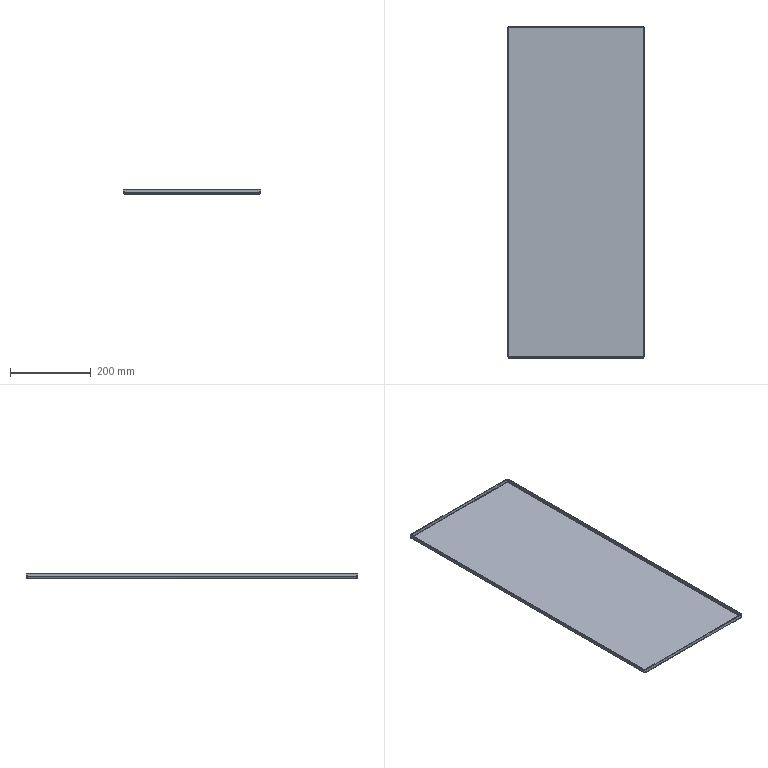Part | SolidWorks | features BaseBody 1 | 1 solid | 38 faces | box 340 x 820 x 10 mm | volume 590888 mm3 | plane 22 | cylinder 8 | spline 8 | commonest cylinder face diameters 1.473 x4 5.473 x4
STEP:
#1=CARTESIAN_POINT('',(-167.263,-407.263,-2.));
#2=VERTEX_POINT('',#1);
#3=CARTESIAN_POINT('',(-167.263,407.263,-2.));
#4=VERTEX_POINT('',#3);
#5=CARTESIAN_POINT('',(-167.263,0.,-2.));
#6=DIRECTION('',(0.,1.,0.));
#7=VECTOR('',#6,1000.);
#8=LINE('',#5,#7);
#9=EDGE_CURVE('',#2,#4,#8,.T.);
#10=ORIENTED_EDGE('',*,*,#9,.T.);
#11=CARTESIAN_POINT('',(167.263,407.263,-2.));
#12=VERTEX_POINT('',#11);
#13=CARTESIAN_POINT('',(0.,407.263,-2.));
#14=DIRECTION('',(1.,0.,0.));
#15=VECTOR('',#14,1000.);
#16=LINE('',#13,#15);
#17=EDGE_CURVE('',#4,#12,#16,.T.);
#18=ORIENTED_EDGE('',*,*,#17,.T.);
#19=CARTESIAN_POINT('',(167.263,-407.263,-2.));
#20=VERTEX_POINT('',#19);
#21=CARTESIAN_POINT('',(167.263,0.,-2.));
#22=DIRECTION('',(0.,-1.,0.));
#23=VECTOR('',#22,1000.);
#24=LINE('',#21,#23);
#25=EDGE_CURVE('',#12,#20,#24,.T.);
#26=ORIENTED_EDGE('',*,*,#25,.T.);
#27=CARTESIAN_POINT('',(0.,-407.263,-2.));
#28=DIRECTION('',(-1.,0.,0.));
#29=VECTOR('',#28,1000.);
#30=LINE('',#27,#29);
#31=EDGE_CURVE('',#20,#2,#30,.T.);
#32=ORIENTED_EDGE('',*,*,#31,.T.);
#33=EDGE_LOOP('',(#10,#18,#26,#32));
#34=FACE_OUTER_BOUND('',#33,.T.);
#35=CARTESIAN_POINT('',(167.263,-407.263,-2.));
#36=DIRECTION('',(0.,0.,-1.));
#37=DIRECTION('',(-1.,0.,0.));
#38=AXIS2_PLACEMENT_3D('',#35,#36,#37);
#39=PLANE('',#38);
#40=ADVANCED_FACE('',(#34),#39,.T.);
#41=CARTESIAN_POINT('',(-167.293,410.,0.7366));
#42=VERTEX_POINT('',#41);
#43=CARTESIAN_POINT('',(-167.293,410.,0.7366));
#44=CARTESIAN_POINT('',(-167.29,410.,0.3784));
#45=CARTESIAN_POINT('',(-167.288,409.929,0.0203));
#46=CARTESIAN_POINT('',(-167.283,409.655,-0.6416));
#47=CARTESIAN_POINT('',(-167.281,409.452,-0.9452));
#48=CARTESIAN_POINT('',(-167.276,408.945,-1.452));
#49=CARTESIAN_POINT('',(-167.273,408.642,-1.655));
#50=CARTESIAN_POINT('',(-167.268,407.98,-1.929));
#51=CARTESIAN_POINT('',(-167.266,407.622,-2.));
#52=CARTESIAN_POINT('',(-167.263,407.263,-2.));
#53=B_SPLINE_CURVE_WITH_KNOTS('',3,(#43,#44,#45,#46,#47,#48,#49,#50,#51,#52),.UNSPECIFIED.,.F.,.F.,(4,2,2,2,4),(0.,0.25,0.5,0.75,1.),.UNSPECIFIED.);
#54=EDGE_CURVE('',#42,#4,#53,.T.);
#55=ORIENTED_EDGE('',*,*,#54,.F.);
#56=CARTESIAN_POINT('',(167.293,410.,0.7366));
#57=VERTEX_POINT('',#56);
#58=CARTESIAN_POINT('',(0.,410.,0.7366));
#59=DIRECTION('',(-1.,0.,0.));
#60=VECTOR('',#59,1000.);
#61=LINE('',#58,#60);
#62=EDGE_CURVE('',#57,#42,#61,.T.);
#63=ORIENTED_EDGE('',*,*,#62,.F.);
#64=CARTESIAN_POINT('',(167.263,407.263,-2.));
#65=CARTESIAN_POINT('',(167.266,407.622,-2.));
#66=CARTESIAN_POINT('',(167.268,407.98,-1.929));
#67=CARTESIAN_POINT('',(167.273,408.642,-1.655));
#68=CARTESIAN_POINT('',(167.276,408.945,-1.452));
#69=CARTESIAN_POINT('',(167.281,409.452,-0.9452));
#70=CARTESIAN_POINT('',(167.283,409.655,-0.6416));
#71=CARTESIAN_POINT('',(167.288,409.929,0.0203));
#72=CARTESIAN_POINT('',(167.29,410.,0.3784));
#73=CARTESIAN_POINT('',(167.293,410.,0.7366));
#74=B_SPLINE_CURVE_WITH_KNOTS('',3,(#64,#65,#66,#67,#68,#69,#70,#71,#72,#73),.UNSPECIFIED.,.F.,.F.,(4,2,2,2,4),(0.,0.25,0.5,0.75,1.),.UNSPECIFIED.);
#75=EDGE_CURVE('',#12,#57,#74,.T.);
#76=ORIENTED_EDGE('',*,*,#75,.F.);
#77=ORIENTED_EDGE('',*,*,#17,.F.);
#78=EDGE_LOOP('',(#55,#63,#76,#77));
#79=FACE_OUTER_BOUND('',#78,.T.);
#80=CARTESIAN_POINT('',(169.3,407.263,0.7366));
#81=DIRECTION('',(-1.,0.,0.));
#82=DIRECTION('',(0.,0.,1.));
#83=AXIS2_PLACEMENT_3D('',#80,#81,#82);
#84=CYLINDRICAL_SURFACE('',#83,2.737);
#85=ADVANCED_FACE('',(#79),#84,.T.);
#86=CARTESIAN_POINT('',(-170.,-407.293,0.7366));
#87=VERTEX_POINT('',#86);
#88=CARTESIAN_POINT('',(-170.,-407.293,0.7366));
#89=CARTESIAN_POINT('',(-170.,-407.29,0.3784));
#90=CARTESIAN_POINT('',(-169.929,-407.288,0.0203));
#91=CARTESIAN_POINT('',(-169.655,-407.283,-0.6416));
#92=CARTESIAN_POINT('',(-169.452,-407.281,-0.9452));
#93=CARTESIAN_POINT('',(-168.945,-407.276,-1.452));
#94=CARTESIAN_POINT('',(-168.642,-407.273,-1.655));
#95=CARTESIAN_POINT('',(-167.98,-407.268,-1.929));
#96=CARTESIAN_POINT('',(-167.622,-407.266,-2.));
#97=CARTESIAN_POINT('',(-167.263,-407.263,-2.));
#98=B_SPLINE_CURVE_WITH_KNOTS('',3,(#88,#89,#90,#91,#92,#93,#94,#95,#96,#97),.UNSPECIFIED.,.F.,.F.,(4,2,2,2,4),(0.,0.25,0.5,0.75,1.),.UNSPECIFIED.);
#99=EDGE_CURVE('',#87,#2,#98,.T.);
#100=ORIENTED_EDGE('',*,*,#99,.F.);
#101=CARTESIAN_POINT('',(-170.,407.293,0.7366));
#102=VERTEX_POINT('',#101);
#103=CARTESIAN_POINT('',(-170.,0.,0.7366));
#104=DIRECTION('',(0.,-1.,0.));
#105=VECTOR('',#104,1000.);
#106=LINE('',#103,#105);
#107=EDGE_CURVE('',#102,#87,#106,.T.);
#108=ORIENTED_EDGE('',*,*,#107,.F.);
#109=CARTESIAN_POINT('',(-167.263,407.263,-2.));
#110=CARTESIAN_POINT('',(-167.622,407.266,-2.));
#111=CARTESIAN_POINT('',(-167.98,407.268,-1.929));
#112=CARTESIAN_POINT('',(-168.642,407.273,-1.655));
#113=CARTESIAN_POINT('',(-168.945,407.276,-1.452));
#114=CARTESIAN_POINT('',(-169.452,407.281,-0.9452));
#115=CARTESIAN_POINT('',(-169.655,407.283,-0.6416));
#116=CARTESIAN_POINT('',(-169.929,407.288,0.0203));
#117=CARTESIAN_POINT('',(-170.,407.29,0.3784));
#118=CARTESIAN_POINT('',(-170.,407.293,0.7366));
#119=B_SPLINE_CURVE_WITH_KNOTS('',3,(#109,#110,#111,#112,#113,#114,#115,#116,#117,#118),.UNSPECIFIED.,.F.,.F.,(4,2,2,2,4),(0.,0.25,0.5,0.75,1.),.UNSPECIFIED.);
#120=EDGE_CURVE('',#4,#102,#119,.T.);
#121=ORIENTED_EDGE('',*,*,#120,.F.);
#122=ORIENTED_EDGE('',*,*,#9,.F.);
#123=EDGE_LOOP('',(#100,#108,#121,#122));
#124=FACE_OUTER_BOUND('',#123,.T.);
#125=CARTESIAN_POINT('',(-167.263,412.18,0.7366));
#126=DIRECTION('',(0.,-1.,0.));
#127=DIRECTION('',(0.,0.,-1.));
#128=AXIS2_PLACEMENT_3D('',#125,#126,#127);
#129=CYLINDRICAL_SURFACE('',#128,2.737);
#130=ADVANCED_FACE('',(#124),#129,.T.);
#131=CARTESIAN_POINT('',(167.293,-410.,0.7366));
#132=VERTEX_POINT('',#131);
#133=CARTESIAN_POINT('',(167.293,-410.,0.7366));
#134=CARTESIAN_POINT('',(167.29,-410.,0.3784));
#135=CARTESIAN_POINT('',(167.288,-409.929,0.0203));
#136=CARTESIAN_POINT('',(167.283,-409.655,-0.6416));
#137=CARTESIAN_POINT('',(167.281,-409.452,-0.9452));
#138=CARTESIAN_POINT('',(167.276,-408.945,-1.452));
#139=CARTESIAN_POINT('',(167.273,-408.642,-1.655));
#140=CARTESIAN_POINT('',(167.268,-407.98,-1.929));
#141=CARTESIAN_POINT('',(167.266,-407.622,-2.));
#142=CARTESIAN_POINT('',(167.263,-407.263,-2.));
#143=B_SPLINE_CURVE_WITH_KNOTS('',3,(#133,#134,#135,#136,#137,#138,#139,#140,#141,#142),.UNSPECIFIED.,.F.,.F.,(4,2,2,2,4),(0.,0.25,0.5,0.75,1.),.UNSPECIFIED.);
#144=EDGE_CURVE('',#132,#20,#143,.T.);
#145=ORIENTED_EDGE('',*,*,#144,.F.);
#146=CARTESIAN_POINT('',(-167.293,-410.,0.7366));
#147=VERTEX_POINT('',#146);
#148=CARTESIAN_POINT('',(0.,-410.,0.7366));
#149=DIRECTION('',(1.,0.,0.));
#150=VECTOR('',#149,1000.);
#151=LINE('',#148,#150);
#152=EDGE_CURVE('',#147,#132,#151,.T.);
#153=ORIENTED_EDGE('',*,*,#152,.F.);
#154=CARTESIAN_POINT('',(-167.263,-407.263,-2.));
#155=CARTESIAN_POINT('',(-167.266,-407.622,-2.));
#156=CARTESIAN_POINT('',(-167.268,-407.98,-1.929));
#157=CARTESIAN_POINT('',(-167.273,-408.642,-1.655));
#158=CARTESIAN_POINT('',(-167.276,-408.945,-1.452));
#159=CARTESIAN_POINT('',(-167.281,-409.452,-0.9452));
#160=CARTESIAN_POINT('',(-167.283,-409.655,-0.6416));
#161=CARTESIAN_POINT('',(-167.288,-409.929,0.0203));
#162=CARTESIAN_POINT('',(-167.29,-410.,0.3784));
#163=CARTESIAN_POINT('',(-167.293,-410.,0.7366));
#164=B_SPLINE_CURVE_WITH_KNOTS('',3,(#154,#155,#156,#157,#158,#159,#160,#161,#162,#163),.UNSPECIFIED.,.F.,.F.,(4,2,2,2,4),(0.,0.25,0.5,0.75,1.),.UNSPECIFIED.);
#165=EDGE_CURVE('',#2,#147,#164,.T.);
#166=ORIENTED_EDGE('',*,*,#165,.F.);
#167=ORIENTED_EDGE('',*,*,#31,.F.);
#168=EDGE_LOOP('',(#145,#153,#166,#167));
#169=FACE_OUTER_BOUND('',#168,.T.);
#170=CARTESIAN_POINT('',(-169.3,-407.263,0.7366));
#171=DIRECTION('',(1.,0.,0.));
#172=DIRECTION('',(0.,0.,-1.));
#173=AXIS2_PLACEMENT_3D('',#170,#171,#172);
#174=CYLINDRICAL_SURFACE('',#173,2.737);
#175=ADVANCED_FACE('',(#169),#174,.T.);
#176=CARTESIAN_POINT('',(170.,407.293,0.7366));
#177=VERTEX_POINT('',#176);
#178=CARTESIAN_POINT('',(170.,407.293,0.7366));
#179=CARTESIAN_POINT('',(170.,407.29,0.3784));
#180=CARTESIAN_POINT('',(169.929,407.288,0.0203));
#181=CARTESIAN_POINT('',(169.655,407.283,-0.6416));
#182=CARTESIAN_POINT('',(169.452,407.281,-0.9452));
#183=CARTESIAN_POINT('',(168.945,407.276,-1.452));
#184=CARTESIAN_POINT('',(168.642,407.273,-1.655));
#185=CARTESIAN_POINT('',(167.98,407.268,-1.929));
#186=CARTESIAN_POINT('',(167.622,407.266,-2.));
#187=CARTESIAN_POINT('',(167.263,407.263,-2.));
#188=B_SPLINE_CURVE_WITH_KNOTS('',3,(#178,#179,#180,#181,#182,#183,#184,#185,#186,#187),.UNSPECIFIED.,.F.,.F.,(4,2,2,2,4),(0.,0.25,0.5,0.75,1.),.UNSPECIFIED.);
#189=EDGE_CURVE('',#177,#12,#188,.T.);
#190=ORIENTED_EDGE('',*,*,#189,.F.);
#191=CARTESIAN_POINT('',(170.,-407.293,0.7366));
#192=VERTEX_POINT('',#191);
#193=CARTESIAN_POINT('',(170.,0.,0.7366));
#194=DIRECTION('',(0.,1.,0.));
#195=VECTOR('',#194,1000.);
#196=LINE('',#193,#195);
#197=EDGE_CURVE('',#192,#177,#196,.T.);
#198=ORIENTED_EDGE('',*,*,#197,.F.);
#199=CARTESIAN_POINT('',(167.263,-407.263,-2.));
#200=CARTESIAN_POINT('',(167.622,-407.266,-2.));
#201=CARTESIAN_POINT('',(167.98,-407.268,-1.929));
#202=CARTESIAN_POINT('',(168.642,-407.273,-1.655));
#203=CARTESIAN_POINT('',(168.945,-407.276,-1.452));
#204=CARTESIAN_POINT('',(169.452,-407.281,-0.9452));
#205=CARTESIAN_POINT('',(169.655,-407.283,-0.6416));
#206=CARTESIAN_POINT('',(169.929,-407.288,0.0203));
#207=CARTESIAN_POINT('',(170.,-407.29,0.3784));
#208=CARTESIAN_POINT('',(170.,-407.293,0.7366));
#209=B_SPLINE_CURVE_WITH_KNOTS('',3,(#199,#200,#201,#202,#203,#204,#205,#206,#207,#208),.UNSPECIFIED.,.F.,.F.,(4,2,2,2,4),(0.,0.25,0.5,0.75,1.),.UNSPECIFIED.);
#210=EDGE_CURVE('',#20,#192,#209,.T.);
#211=ORIENTED_EDGE('',*,*,#210,.F.);
#212=ORIENTED_EDGE('',*,*,#25,.F.);
#213=EDGE_LOOP('',(#190,#198,#211,#212));
#214=FACE_OUTER_BOUND('',#213,.T.);
#215=CARTESIAN_POINT('',(167.263,-412.18,0.7366));
#216=DIRECTION('',(0.,1.,0.));
#217=DIRECTION('',(0.,0.,1.));
#218=AXIS2_PLACEMENT_3D('',#215,#216,#217);
#219=CYLINDRICAL_SURFACE('',#218,2.737);
#220=ADVANCED_FACE('',(#214),#219,.T.);
#221=CARTESIAN_POINT('',(-167.293,408.,0.7366));
#222=VERTEX_POINT('',#221);
#223=CARTESIAN_POINT('',(-167.293,409.,0.7366));
#224=DIRECTION('',(0.,-1.,0.));
#225=VECTOR('',#224,1000.);
#226=LINE('',#223,#225);
#227=EDGE_CURVE('',#42,#222,#226,.T.);
#228=ORIENTED_EDGE('',*,*,#227,.F.);
#229=ORIENTED_EDGE('',*,*,#54,.T.);
#230=CARTESIAN_POINT('',(-167.263,407.263,0.));
#231=VERTEX_POINT('',#230);
#232=CARTESIAN_POINT('',(-167.263,407.263,-1.));
#233=DIRECTION('',(0.,0.,-1.));
#234=VECTOR('',#233,1000.);
#235=LINE('',#232,#234);
#236=EDGE_CURVE('',#231,#4,#235,.T.);
#237=ORIENTED_EDGE('',*,*,#236,.F.);
#238=CARTESIAN_POINT('',(-167.293,408.,0.7366));
#239=CARTESIAN_POINT('',(-167.288,408.,0.5438));
#240=CARTESIAN_POINT('',(-167.283,407.921,0.3521));
#241=CARTESIAN_POINT('',(-167.273,407.648,0.07939));
#242=CARTESIAN_POINT('',(-167.268,407.456,0.));
#243=CARTESIAN_POINT('',(-167.263,407.263,0.));
#244=B_SPLINE_CURVE_WITH_KNOTS('',3,(#238,#239,#240,#241,#242,#243),.UNSPECIFIED.,.F.,.F.,(4,2,4),(0.,0.5,1.),.UNSPECIFIED.);
#245=EDGE_CURVE('',#222,#231,#244,.T.);
#246=ORIENTED_EDGE('',*,*,#245,.F.);
#247=EDGE_LOOP('',(#228,#229,#237,#246));
#248=FACE_OUTER_BOUND('',#247,.T.);
#249=CARTESIAN_POINT('',(-167.293,410.012,0.7366));
#250=CARTESIAN_POINT('',(-167.29,410.012,0.3767));
#251=CARTESIAN_POINT('',(-167.288,409.941,0.01711));
#252=CARTESIAN_POINT('',(-167.283,409.665,-0.6477));
#253=CARTESIAN_POINT('',(-167.281,409.462,-0.9527));
#254=CARTESIAN_POINT('',(-167.276,408.953,-1.462));
#255=CARTESIAN_POINT('',(-167.273,408.648,-1.665));
#256=CARTESIAN_POINT('',(-167.268,407.983,-1.941));
#257=CARTESIAN_POINT('',(-167.266,407.623,-2.012));
#258=CARTESIAN_POINT('',(-167.263,407.263,-2.012));
#259=CARTESIAN_POINT('',(-167.293,410.,0.7366));
#260=CARTESIAN_POINT('',(-167.29,410.,0.3783));
#261=CARTESIAN_POINT('',(-167.288,409.929,0.0203));
#262=CARTESIAN_POINT('',(-167.283,409.655,-0.6416));
#263=CARTESIAN_POINT('',(-167.281,409.452,-0.9452));
#264=CARTESIAN_POINT('',(-167.276,408.945,-1.452));
#265=CARTESIAN_POINT('',(-167.273,408.642,-1.655));
#266=CARTESIAN_POINT('',(-167.268,407.98,-1.929));
#267=CARTESIAN_POINT('',(-167.266,407.622,-2.));
#268=CARTESIAN_POINT('',(-167.263,407.263,-2.));
#269=CARTESIAN_POINT('',(-167.293,408.,0.7366));
#270=CARTESIAN_POINT('',(-167.29,408.,0.6402));
#271=CARTESIAN_POINT('',(-167.288,407.981,0.5438));
#272=CARTESIAN_POINT('',(-167.283,407.907,0.3656));
#273=CARTESIAN_POINT('',(-167.281,407.852,0.2839));
#274=CARTESIAN_POINT('',(-167.276,407.716,0.1476));
#275=CARTESIAN_POINT('',(-167.273,407.634,0.09297));
#276=CARTESIAN_POINT('',(-167.268,407.456,0.01917));
#277=CARTESIAN_POINT('',(-167.266,407.36,0.));
#278=CARTESIAN_POINT('',(-167.263,407.263,0.));
#279=CARTESIAN_POINT('',(-167.293,407.988,0.7366));
#280=CARTESIAN_POINT('',(-167.29,407.988,0.6417));
#281=CARTESIAN_POINT('',(-167.288,407.969,0.5469));
#282=CARTESIAN_POINT('',(-167.283,407.897,0.3717));
#283=CARTESIAN_POINT('',(-167.281,407.843,0.2913));
#284=CARTESIAN_POINT('',(-167.276,407.709,0.1572));
#285=CARTESIAN_POINT('',(-167.273,407.628,0.1035));
#286=CARTESIAN_POINT('',(-167.268,407.453,0.03088));
#287=CARTESIAN_POINT('',(-167.266,407.358,0.01202));
#288=CARTESIAN_POINT('',(-167.263,407.263,0.01202));
#289=B_SPLINE_SURFACE_WITH_KNOTS('',1,3,((#249,#250,#251,#252,#253,#254,#255,#256,#257,#258),(#259,#260,#261,#262,#263,#264,#265,#266,#267,#268),(#269,#270,#271,#272,#273,#274,#275,#276,#277,#278),(#279,#280,#281,#282,#283,#284,#285,#286,#287,#288)),.UNSPECIFIED.,.F.,.F.,.F.,(2,1,1,2),(4,2,2,2,4),(-0.006096,0.,1.,1.006),(0.,0.25,0.5,0.75,1.),.UNSPECIFIED.);
#290=ADVANCED_FACE('',(#248),#289,.F.);
#291=CARTESIAN_POINT('',(-167.293,410.,8.));
#292=VERTEX_POINT('',#291);
#293=CARTESIAN_POINT('',(-167.293,410.,4.368));
#294=DIRECTION('',(0.,0.,-1.));
#295=VECTOR('',#294,1000.);
#296=LINE('',#293,#295);
#297=EDGE_CURVE('',#292,#42,#296,.T.);
#298=ORIENTED_EDGE('',*,*,#297,.F.);
#299=CARTESIAN_POINT('',(167.293,410.,8.));
#300=VERTEX_POINT('',#299);
#301=CARTESIAN_POINT('',(0.,410.,8.));
#302=DIRECTION('',(-1.,0.,0.));
#303=VECTOR('',#302,1000.);
#304=LINE('',#301,#303);
#305=EDGE_CURVE('',#300,#292,#304,.T.);
#306=ORIENTED_EDGE('',*,*,#305,.F.);
#307=CARTESIAN_POINT('',(167.293,410.,4.368));
#308=DIRECTION('',(0.,0.,1.));
#309=VECTOR('',#308,1000.);
#310=LINE('',#307,#309);
#311=EDGE_CURVE('',#57,#300,#310,.T.);
#312=ORIENTED_EDGE('',*,*,#311,.F.);
#313=ORIENTED_EDGE('',*,*,#62,.T.);
#314=EDGE_LOOP('',(#298,#306,#312,#313));
#315=FACE_OUTER_BOUND('',#314,.T.);
#316=CARTESIAN_POINT('',(-167.293,410.,8.));
#317=DIRECTION('',(0.,-1.,0.));
#318=DIRECTION('',(0.,0.,-1.));
#319=AXIS2_PLACEMENT_3D('',#316,#317,#318);
#320=PLANE('',#319);
#321=ADVANCED_FACE('',(#315),#320,.F.);
#322=CARTESIAN_POINT('',(167.263,407.263,0.));
#323=VERTEX_POINT('',#322);
#324=CARTESIAN_POINT('',(167.293,408.,0.7366));
#325=VERTEX_POINT('',#324);
#326=CARTESIAN_POINT('',(167.263,407.263,0.));
#327=CARTESIAN_POINT('',(167.268,407.456,0.));
#328=CARTESIAN_POINT('',(167.273,407.648,0.07939));
#329=CARTESIAN_POINT('',(167.283,407.921,0.3521));
#330=CARTESIAN_POINT('',(167.288,408.,0.5438));
#331=CARTESIAN_POINT('',(167.293,408.,0.7366));
#332=B_SPLINE_CURVE_WITH_KNOTS('',3,(#326,#327,#328,#329,#330,#331),.UNSPECIFIED.,.F.,.F.,(4,2,4),(0.,0.5,1.),.UNSPECIFIED.);
#333=EDGE_CURVE('',#323,#325,#332,.T.);
#334=ORIENTED_EDGE('',*,*,#333,.F.);
#335=CARTESIAN_POINT('',(167.263,407.263,-1.));
#336=DIRECTION('',(0.,0.,1.));
#337=VECTOR('',#336,1000.);
#338=LINE('',#335,#337);
#339=EDGE_CURVE('',#12,#323,#338,.T.);
#340=ORIENTED_EDGE('',*,*,#339,.F.);
#341=ORIENTED_EDGE('',*,*,#75,.T.);
#342=CARTESIAN_POINT('',(167.293,409.,0.7366));
#343=DIRECTION('',(0.,1.,0.));
#344=VECTOR('',#343,1000.);
#345=LINE('',#342,#344);
#346=EDGE_CURVE('',#325,#57,#345,.T.);
#347=ORIENTED_EDGE('',*,*,#346,.F.);
#348=EDGE_LOOP('',(#334,#340,#341,#347));
#349=FACE_OUTER_BOUND('',#348,.T.);
#350=CARTESIAN_POINT('',(167.263,407.263,-2.012));
#351=CARTESIAN_POINT('',(167.266,407.623,-2.012));
#352=CARTESIAN_POINT('',(167.268,407.983,-1.941));
#353=CARTESIAN_POINT('',(167.273,408.648,-1.665));
#354=CARTESIAN_POINT('',(167.276,408.953,-1.462));
#355=CARTESIAN_POINT('',(167.281,409.462,-0.9527));
#356=CARTESIAN_POINT('',(167.283,409.665,-0.6477));
#357=CARTESIAN_POINT('',(167.288,409.941,0.01711));
#358=CARTESIAN_POINT('',(167.29,410.012,0.3767));
#359=CARTESIAN_POINT('',(167.293,410.012,0.7366));
#360=CARTESIAN_POINT('',(167.263,407.263,-2.));
#361=CARTESIAN_POINT('',(167.266,407.622,-2.));
#362=CARTESIAN_POINT('',(167.268,407.98,-1.929));
#363=CARTESIAN_POINT('',(167.273,408.642,-1.655));
#364=CARTESIAN_POINT('',(167.276,408.945,-1.452));
#365=CARTESIAN_POINT('',(167.281,409.452,-0.9452));
#366=CARTESIAN_POINT('',(167.283,409.655,-0.6416));
#367=CARTESIAN_POINT('',(167.288,409.929,0.0203));
#368=CARTESIAN_POINT('',(167.29,410.,0.3783));
#369=CARTESIAN_POINT('',(167.293,410.,0.7366));
#370=CARTESIAN_POINT('',(167.263,407.263,0.));
#371=CARTESIAN_POINT('',(167.266,407.36,0.));
#372=CARTESIAN_POINT('',(167.268,407.456,0.01917));
#373=CARTESIAN_POINT('',(167.273,407.634,0.09297));
#374=CARTESIAN_POINT('',(167.276,407.716,0.1476));
#375=CARTESIAN_POINT('',(167.281,407.852,0.2839));
#376=CARTESIAN_POINT('',(167.283,407.907,0.3656));
#377=CARTESIAN_POINT('',(167.288,407.981,0.5438));
#378=CARTESIAN_POINT('',(167.29,408.,0.6402));
#379=CARTESIAN_POINT('',(167.293,408.,0.7366));
#380=CARTESIAN_POINT('',(167.263,407.263,0.01202));
#381=CARTESIAN_POINT('',(167.266,407.358,0.01202));
#382=CARTESIAN_POINT('',(167.268,407.453,0.03088));
#383=CARTESIAN_POINT('',(167.273,407.628,0.1035));
#384=CARTESIAN_POINT('',(167.276,407.709,0.1572));
#385=CARTESIAN_POINT('',(167.281,407.843,0.2913));
#386=CARTESIAN_POINT('',(167.283,407.897,0.3717));
#387=CARTESIAN_POINT('',(167.288,407.969,0.5469));
#388=CARTESIAN_POINT('',(167.29,407.988,0.6417));
#389=CARTESIAN_POINT('',(167.293,407.988,0.7366));
#390=B_SPLINE_SURFACE_WITH_KNOTS('',1,3,((#350,#351,#352,#353,#354,#355,#356,#357,#358,#359),(#360,#361,#362,#363,#364,#365,#366,#367,#368,#369),(#370,#371,#372,#373,#374,#375,#376,#377,#378,#379),(#380,#381,#382,#383,#384,#385,#386,#387,#388,#389)),.UNSPECIFIED.,.F.,.F.,.F.,(2,1,1,2),(4,2,2,2,4),(-0.006096,0.,1.,1.006),(0.,0.25,0.5,0.75,1.),.UNSPECIFIED.);
#391=ADVANCED_FACE('',(#349),#390,.F.);
#392=CARTESIAN_POINT('',(-168.,-407.293,0.7366));
#393=VERTEX_POINT('',#392);
#394=CARTESIAN_POINT('',(-169.,-407.293,0.7366));
#395=DIRECTION('',(1.,0.,0.));
#396=VECTOR('',#395,1000.);
#397=LINE('',#394,#396);
#398=EDGE_CURVE('',#87,#393,#397,.T.);
#399=ORIENTED_EDGE('',*,*,#398,.F.);
#400=ORIENTED_EDGE('',*,*,#99,.T.);
#401=CARTESIAN_POINT('',(-167.263,-407.263,0.));
#402=VERTEX_POINT('',#401);
#403=CARTESIAN_POINT('',(-167.263,-407.263,-1.));
#404=DIRECTION('',(0.,0.,-1.));
#405=VECTOR('',#404,1000.);
#406=LINE('',#403,#405);
#407=EDGE_CURVE('',#402,#2,#406,.T.);
#408=ORIENTED_EDGE('',*,*,#407,.F.);
#409=CARTESIAN_POINT('',(-168.,-407.293,0.7366));
#410=CARTESIAN_POINT('',(-168.,-407.288,0.5438));
#411=CARTESIAN_POINT('',(-167.921,-407.283,0.3521));
#412=CARTESIAN_POINT('',(-167.648,-407.273,0.07939));
#413=CARTESIAN_POINT('',(-167.456,-407.268,0.));
#414=CARTESIAN_POINT('',(-167.263,-407.263,0.));
#415=B_SPLINE_CURVE_WITH_KNOTS('',3,(#409,#410,#411,#412,#413,#414),.UNSPECIFIED.,.F.,.F.,(4,2,4),(0.,0.5,1.),.UNSPECIFIED.);
#416=EDGE_CURVE('',#393,#402,#415,.T.);
#417=ORIENTED_EDGE('',*,*,#416,.F.);
#418=EDGE_LOOP('',(#399,#400,#408,#417));
#419=FACE_OUTER_BOUND('',#418,.T.);
#420=CARTESIAN_POINT('',(-170.012,-407.293,0.7366));
#421=CARTESIAN_POINT('',(-170.012,-407.29,0.3767));
#422=CARTESIAN_POINT('',(-169.941,-407.288,0.01711));
#423=CARTESIAN_POINT('',(-169.665,-407.283,-0.6477));
#424=CARTESIAN_POINT('',(-169.462,-407.281,-0.9527));
#425=CARTESIAN_POINT('',(-168.953,-407.276,-1.462));
#426=CARTESIAN_POINT('',(-168.648,-407.273,-1.665));
#427=CARTESIAN_POINT('',(-167.983,-407.268,-1.941));
#428=CARTESIAN_POINT('',(-167.623,-407.266,-2.012));
#429=CARTESIAN_POINT('',(-167.263,-407.263,-2.012));
#430=CARTESIAN_POINT('',(-170.,-407.293,0.7366));
#431=CARTESIAN_POINT('',(-170.,-407.29,0.3783));
#432=CARTESIAN_POINT('',(-169.929,-407.288,0.0203));
#433=CARTESIAN_POINT('',(-169.655,-407.283,-0.6416));
#434=CARTESIAN_POINT('',(-169.452,-407.281,-0.9452));
#435=CARTESIAN_POINT('',(-168.945,-407.276,-1.452));
#436=CARTESIAN_POINT('',(-168.642,-407.273,-1.655));
#437=CARTESIAN_POINT('',(-167.98,-407.268,-1.929));
#438=CARTESIAN_POINT('',(-167.622,-407.266,-2.));
#439=CARTESIAN_POINT('',(-167.263,-407.263,-2.));
#440=CARTESIAN_POINT('',(-168.,-407.293,0.7366));
#441=CARTESIAN_POINT('',(-168.,-407.29,0.6402));
#442=CARTESIAN_POINT('',(-167.981,-407.288,0.5438));
#443=CARTESIAN_POINT('',(-167.907,-407.283,0.3656));
#444=CARTESIAN_POINT('',(-167.852,-407.281,0.2839));
#445=CARTESIAN_POINT('',(-167.716,-407.276,0.1476));
#446=CARTESIAN_POINT('',(-167.634,-407.273,0.09297));
#447=CARTESIAN_POINT('',(-167.456,-407.268,0.01917));
#448=CARTESIAN_POINT('',(-167.36,-407.266,0.));
#449=CARTESIAN_POINT('',(-167.263,-407.263,0.));
#450=CARTESIAN_POINT('',(-167.988,-407.293,0.7366));
#451=CARTESIAN_POINT('',(-167.988,-407.29,0.6417));
#452=CARTESIAN_POINT('',(-167.969,-407.288,0.5469));
#453=CARTESIAN_POINT('',(-167.897,-407.283,0.3717));
#454=CARTESIAN_POINT('',(-167.843,-407.281,0.2913));
#455=CARTESIAN_POINT('',(-167.709,-407.276,0.1572));
#456=CARTESIAN_POINT('',(-167.628,-407.273,0.1035));
#457=CARTESIAN_POINT('',(-167.453,-407.268,0.03088));
#458=CARTESIAN_POINT('',(-167.358,-407.266,0.01202));
#459=CARTESIAN_POINT('',(-167.263,-407.263,0.01202));
#460=B_SPLINE_SURFACE_WITH_KNOTS('',1,3,((#420,#421,#422,#423,#424,#425,#426,#427,#428,#429),(#430,#431,#432,#433,#434,#435,#436,#437,#438,#439),(#440,#441,#442,#443,#444,#445,#446,#447,#448,#449),(#450,#451,#452,#453,#454,#455,#456,#457,#458,#459)),.UNSPECIFIED.,.F.,.F.,.F.,(2,1,1,2),(4,2,2,2,4),(-0.006096,0.,1.,1.006),(0.,0.25,0.5,0.75,1.),.UNSPECIFIED.);
#461=ADVANCED_FACE('',(#419),#460,.F.);
#462=CARTESIAN_POINT('',(-170.,-407.293,8.));
#463=VERTEX_POINT('',#462);
#464=CARTESIAN_POINT('',(-170.,-407.293,4.368));
#465=DIRECTION('',(0.,0.,-1.));
#466=VECTOR('',#465,1000.);
#467=LINE('',#464,#466);
#468=EDGE_CURVE('',#463,#87,#467,.T.);
#469=ORIENTED_EDGE('',*,*,#468,.F.);
#470=CARTESIAN_POINT('',(-170.,407.293,8.));
#471=VERTEX_POINT('',#470);
#472=CARTESIAN_POINT('',(-170.,0.,8.));
#473=DIRECTION('',(0.,-1.,0.));
#474=VECTOR('',#473,1000.);
#475=LINE('',#472,#474);
#476=EDGE_CURVE('',#471,#463,#475,.T.);
#477=ORIENTED_EDGE('',*,*,#476,.F.);
#478=CARTESIAN_POINT('',(-170.,407.293,4.368));
#479=DIRECTION('',(0.,0.,1.));
#480=VECTOR('',#479,1000.);
#481=LINE('',#478,#480);
#482=EDGE_CURVE('',#102,#471,#481,.T.);
#483=ORIENTED_EDGE('',*,*,#482,.F.);
#484=ORIENTED_EDGE('',*,*,#107,.T.);
#485=EDGE_LOOP('',(#469,#477,#483,#484));
#486=FACE_OUTER_BOUND('',#485,.T.);
#487=CARTESIAN_POINT('',(-170.,-407.293,8.));
#488=DIRECTION('',(1.,0.,0.));
#489=DIRECTION('',(0.,0.,-1.));
#490=AXIS2_PLACEMENT_3D('',#487,#488,#489);
#491=PLANE('',#490);
#492=ADVANCED_FACE('',(#486),#491,.F.);
#493=CARTESIAN_POINT('',(-168.,407.293,0.7366));
#494=VERTEX_POINT('',#493);
#495=CARTESIAN_POINT('',(-167.263,407.263,0.));
#496=CARTESIAN_POINT('',(-167.456,407.268,0.));
#497=CARTESIAN_POINT('',(-167.648,407.273,0.07939));
#498=CARTESIAN_POINT('',(-167.921,407.283,0.3521));
#499=CARTESIAN_POINT('',(-168.,407.288,0.5438));
#500=CARTESIAN_POINT('',(-168.,407.293,0.7366));
#501=B_SPLINE_CURVE_WITH_KNOTS('',3,(#495,#496,#497,#498,#499,#500),.UNSPECIFIED.,.F.,.F.,(4,2,4),(0.,0.5,1.),.UNSPECIFIED.);
#502=EDGE_CURVE('',#231,#494,#501,.T.);
#503=ORIENTED_EDGE('',*,*,#502,.F.);
#504=ORIENTED_EDGE('',*,*,#236,.T.);
#505=ORIENTED_EDGE('',*,*,#120,.T.);
#506=CARTESIAN_POINT('',(-169.,407.293,0.7366));
#507=DIRECTION('',(-1.,0.,0.));
#508=VECTOR('',#507,1000.);
#509=LINE('',#506,#508);
#510=EDGE_CURVE('',#494,#102,#509,.T.);
#511=ORIENTED_EDGE('',*,*,#510,.F.);
#512=EDGE_LOOP('',(#503,#504,#505,#511));
#513=FACE_OUTER_BOUND('',#512,.T.);
#514=CARTESIAN_POINT('',(-167.263,407.263,-2.012));
#515=CARTESIAN_POINT('',(-167.623,407.266,-2.012));
#516=CARTESIAN_POINT('',(-167.983,407.268,-1.941));
#517=CARTESIAN_POINT('',(-168.648,407.273,-1.665));
#518=CARTESIAN_POINT('',(-168.953,407.276,-1.462));
#519=CARTESIAN_POINT('',(-169.462,407.281,-0.9527));
#520=CARTESIAN_POINT('',(-169.665,407.283,-0.6477));
#521=CARTESIAN_POINT('',(-169.941,407.288,0.01711));
#522=CARTESIAN_POINT('',(-170.012,407.29,0.3767));
#523=CARTESIAN_POINT('',(-170.012,407.293,0.7366));
#524=CARTESIAN_POINT('',(-167.263,407.263,-2.));
#525=CARTESIAN_POINT('',(-167.622,407.266,-2.));
#526=CARTESIAN_POINT('',(-167.98,407.268,-1.929));
#527=CARTESIAN_POINT('',(-168.642,407.273,-1.655));
#528=CARTESIAN_POINT('',(-168.945,407.276,-1.452));
#529=CARTESIAN_POINT('',(-169.452,407.281,-0.9452));
#530=CARTESIAN_POINT('',(-169.655,407.283,-0.6416));
#531=CARTESIAN_POINT('',(-169.929,407.288,0.0203));
#532=CARTESIAN_POINT('',(-170.,407.29,0.3783));
#533=CARTESIAN_POINT('',(-170.,407.293,0.7366));
#534=CARTESIAN_POINT('',(-167.263,407.263,0.));
#535=CARTESIAN_POINT('',(-167.36,407.266,0.));
#536=CARTESIAN_POINT('',(-167.456,407.268,0.01917));
#537=CARTESIAN_POINT('',(-167.634,407.273,0.09297));
#538=CARTESIAN_POINT('',(-167.716,407.276,0.1476));
#539=CARTESIAN_POINT('',(-167.852,407.281,0.2839));
#540=CARTESIAN_POINT('',(-167.907,407.283,0.3656));
#541=CARTESIAN_POINT('',(-167.981,407.288,0.5438));
#542=CARTESIAN_POINT('',(-168.,407.29,0.6402));
#543=CARTESIAN_POINT('',(-168.,407.293,0.7366));
#544=CARTESIAN_POINT('',(-167.263,407.263,0.01202));
#545=CARTESIAN_POINT('',(-167.358,407.266,0.01202));
#546=CARTESIAN_POINT('',(-167.453,407.268,0.03088));
#547=CARTESIAN_POINT('',(-167.628,407.273,0.1035));
#548=CARTESIAN_POINT('',(-167.709,407.276,0.1572));
#549=CARTESIAN_POINT('',(-167.843,407.281,0.2913));
#550=CARTESIAN_POINT('',(-167.897,407.283,0.3717));
#551=CARTESIAN_POINT('',(-167.969,407.288,0.5469));
#552=CARTESIAN_POINT('',(-167.988,407.29,0.6417));
#553=CARTESIAN_POINT('',(-167.988,407.293,0.7366));
#554=B_SPLINE_SURFACE_WITH_KNOTS('',1,3,((#514,#515,#516,#517,#518,#519,#520,#521,#522,#523),(#524,#525,#526,#527,#528,#529,#530,#531,#532,#533),(#534,#535,#536,#537,#538,#539,#540,#541,#542,#543),(#544,#545,#546,#547,#548,#549,#550,#551,#552,#553)),.UNSPECIFIED.,.F.,.F.,.F.,(2,1,1,2),(4,2,2,2,4),(-0.006096,0.,1.,1.006),(0.,0.25,0.5,0.75,1.),.UNSPECIFIED.);
#555=ADVANCED_FACE('',(#513),#554,.F.);
#556=CARTESIAN_POINT('',(167.293,-408.,0.7366));
#557=VERTEX_POINT('',#556);
#558=CARTESIAN_POINT('',(167.293,-409.,0.7366));
#559=DIRECTION('',(0.,1.,0.));
#560=VECTOR('',#559,1000.);
#561=LINE('',#558,#560);
#562=EDGE_CURVE('',#132,#557,#561,.T.);
#563=ORIENTED_EDGE('',*,*,#562,.F.);
#564=ORIENTED_EDGE('',*,*,#144,.T.);
#565=CARTESIAN_POINT('',(167.263,-407.263,0.));
#566=VERTEX_POINT('',#565);
#567=CARTESIAN_POINT('',(167.263,-407.263,-1.));
#568=DIRECTION('',(0.,0.,-1.));
#569=VECTOR('',#568,1000.);
#570=LINE('',#567,#569);
#571=EDGE_CURVE('',#566,#20,#570,.T.);
#572=ORIENTED_EDGE('',*,*,#571,.F.);
#573=CARTESIAN_POINT('',(167.293,-408.,0.7366));
#574=CARTESIAN_POINT('',(167.288,-408.,0.5438));
#575=CARTESIAN_POINT('',(167.283,-407.921,0.3521));
#576=CARTESIAN_POINT('',(167.273,-407.648,0.07939));
#577=CARTESIAN_POINT('',(167.268,-407.456,0.));
#578=CARTESIAN_POINT('',(167.263,-407.263,0.));
#579=B_SPLINE_CURVE_WITH_KNOTS('',3,(#573,#574,#575,#576,#577,#578),.UNSPECIFIED.,.F.,.F.,(4,2,4),(0.,0.5,1.),.UNSPECIFIED.);
#580=EDGE_CURVE('',#557,#566,#579,.T.);
#581=ORIENTED_EDGE('',*,*,#580,.F.);
#582=EDGE_LOOP('',(#563,#564,#572,#581));
#583=FACE_OUTER_BOUND('',#582,.T.);
#584=CARTESIAN_POINT('',(167.293,-410.012,0.7366));
#585=CARTESIAN_POINT('',(167.29,-410.012,0.3767));
#586=CARTESIAN_POINT('',(167.288,-409.941,0.01711));
#587=CARTESIAN_POINT('',(167.283,-409.665,-0.6477));
#588=CARTESIAN_POINT('',(167.281,-409.462,-0.9527));
#589=CARTESIAN_POINT('',(167.276,-408.953,-1.462));
#590=CARTESIAN_POINT('',(167.273,-408.648,-1.665));
#591=CARTESIAN_POINT('',(167.268,-407.983,-1.941));
#592=CARTESIAN_POINT('',(167.266,-407.623,-2.012));
#593=CARTESIAN_POINT('',(167.263,-407.263,-2.012));
#594=CARTESIAN_POINT('',(167.293,-410.,0.7366));
#595=CARTESIAN_POINT('',(167.29,-410.,0.3783));
#596=CARTESIAN_POINT('',(167.288,-409.929,0.0203));
#597=CARTESIAN_POINT('',(167.283,-409.655,-0.6416));
#598=CARTESIAN_POINT('',(167.281,-409.452,-0.9452));
#599=CARTESIAN_POINT('',(167.276,-408.945,-1.452));
#600=CARTESIAN_POINT('',(167.273,-408.642,-1.655));
#601=CARTESIAN_POINT('',(167.268,-407.98,-1.929));
#602=CARTESIAN_POINT('',(167.266,-407.622,-2.));
#603=CARTESIAN_POINT('',(167.263,-407.263,-2.));
#604=CARTESIAN_POINT('',(167.293,-408.,0.7366));
#605=CARTESIAN_POINT('',(167.29,-408.,0.6402));
#606=CARTESIAN_POINT('',(167.288,-407.981,0.5438));
#607=CARTESIAN_POINT('',(167.283,-407.907,0.3656));
#608=CARTESIAN_POINT('',(167.281,-407.852,0.2839));
#609=CARTESIAN_POINT('',(167.276,-407.716,0.1476));
#610=CARTESIAN_POINT('',(167.273,-407.634,0.09297));
#611=CARTESIAN_POINT('',(167.268,-407.456,0.01917));
#612=CARTESIAN_POINT('',(167.266,-407.36,0.));
#613=CARTESIAN_POINT('',(167.263,-407.263,0.));
#614=CARTESIAN_POINT('',(167.293,-407.988,0.7366));
#615=CARTESIAN_POINT('',(167.29,-407.988,0.6417));
#616=CARTESIAN_POINT('',(167.288,-407.969,0.5469));
#617=CARTESIAN_POINT('',(167.283,-407.897,0.3717));
#618=CARTESIAN_POINT('',(167.281,-407.843,0.2913));
#619=CARTESIAN_POINT('',(167.276,-407.709,0.1572));
#620=CARTESIAN_POINT('',(167.273,-407.628,0.1035));
#621=CARTESIAN_POINT('',(167.268,-407.453,0.03088));
#622=CARTESIAN_POINT('',(167.266,-407.358,0.01202));
#623=CARTESIAN_POINT('',(167.263,-407.263,0.01202));
#624=B_SPLINE_SURFACE_WITH_KNOTS('',1,3,((#584,#585,#586,#587,#588,#589,#590,#591,#592,#593),(#594,#595,#596,#597,#598,#599,#600,#601,#602,#603),(#604,#605,#606,#607,#608,#609,#610,#611,#612,#613),(#614,#615,#616,#617,#618,#619,#620,#621,#622,#623)),.UNSPECIFIED.,.F.,.F.,.F.,(2,1,1,2),(4,2,2,2,4),(-0.006096,0.,1.,1.006),(0.,0.25,0.5,0.75,1.),.UNSPECIFIED.);
#625=ADVANCED_FACE('',(#583),#624,.F.);
#626=CARTESIAN_POINT('',(167.293,-410.,8.));
#627=VERTEX_POINT('',#626);
#628=CARTESIAN_POINT('',(167.293,-410.,4.368));
#629=DIRECTION('',(0.,0.,-1.));
#630=VECTOR('',#629,1000.);
#631=LINE('',#628,#630);
#632=EDGE_CURVE('',#627,#132,#631,.T.);
#633=ORIENTED_EDGE('',*,*,#632,.F.);
#634=CARTESIAN_POINT('',(-167.293,-410.,8.));
#635=VERTEX_POINT('',#634);
#636=CARTESIAN_POINT('',(0.,-410.,8.));
#637=DIRECTION('',(1.,0.,0.));
#638=VECTOR('',#637,1000.);
#639=LINE('',#636,#638);
#640=EDGE_CURVE('',#635,#627,#639,.T.);
#641=ORIENTED_EDGE('',*,*,#640,.F.);
#642=CARTESIAN_POINT('',(-167.293,-410.,4.368));
#643=DIRECTION('',(0.,0.,1.));
#644=VECTOR('',#643,1000.);
#645=LINE('',#642,#644);
#646=EDGE_CURVE('',#147,#635,#645,.T.);
#647=ORIENTED_EDGE('',*,*,#646,.F.);
#648=ORIENTED_EDGE('',*,*,#152,.T.);
#649=EDGE_LOOP('',(#633,#641,#647,#648));
#650=FACE_OUTER_BOUND('',#649,.T.);
#651=CARTESIAN_POINT('',(-167.293,-410.,0.7366));
#652=DIRECTION('',(0.,1.,0.));
#653=DIRECTION('',(0.,0.,1.));
#654=AXIS2_PLACEMENT_3D('',#651,#652,#653);
#655=PLANE('',#654);
#656=ADVANCED_FACE('',(#650),#655,.F.);
#657=CARTESIAN_POINT('',(-167.293,-408.,0.7366));
#658=VERTEX_POINT('',#657);
#659=CARTESIAN_POINT('',(-167.263,-407.263,0.));
#660=CARTESIAN_POINT('',(-167.268,-407.456,0.));
#661=CARTESIAN_POINT('',(-167.273,-407.648,0.07939));
#662=CARTESIAN_POINT('',(-167.283,-407.921,0.3521));
#663=CARTESIAN_POINT('',(-167.288,-408.,0.5438));
#664=CARTESIAN_POINT('',(-167.293,-408.,0.7366));
#665=B_SPLINE_CURVE_WITH_KNOTS('',3,(#659,#660,#661,#662,#663,#664),.UNSPECIFIED.,.F.,.F.,(4,2,4),(0.,0.5,1.),.UNSPECIFIED.);
#666=EDGE_CURVE('',#402,#658,#665,.T.);
#667=ORIENTED_EDGE('',*,*,#666,.F.);
#668=ORIENTED_EDGE('',*,*,#407,.T.);
#669=ORIENTED_EDGE('',*,*,#165,.T.);
#670=CARTESIAN_POINT('',(-167.293,-409.,0.7366));
#671=DIRECTION('',(0.,-1.,0.));
#672=VECTOR('',#671,1000.);
#673=LINE('',#670,#672);
#674=EDGE_CURVE('',#658,#147,#673,.T.);
#675=ORIENTED_EDGE('',*,*,#674,.F.);
#676=EDGE_LOOP('',(#667,#668,#669,#675));
#677=FACE_OUTER_BOUND('',#676,.T.);
#678=CARTESIAN_POINT('',(-167.263,-407.263,-2.012));
#679=CARTESIAN_POINT('',(-167.266,-407.623,-2.012));
#680=CARTESIAN_POINT('',(-167.268,-407.983,-1.941));
#681=CARTESIAN_POINT('',(-167.273,-408.648,-1.665));
#682=CARTESIAN_POINT('',(-167.276,-408.953,-1.462));
#683=CARTESIAN_POINT('',(-167.281,-409.462,-0.9527));
#684=CARTESIAN_POINT('',(-167.283,-409.665,-0.6477));
#685=CARTESIAN_POINT('',(-167.288,-409.941,0.01711));
#686=CARTESIAN_POINT('',(-167.29,-410.012,0.3767));
#687=CARTESIAN_POINT('',(-167.293,-410.012,0.7366));
#688=CARTESIAN_POINT('',(-167.263,-407.263,-2.));
#689=CARTESIAN_POINT('',(-167.266,-407.622,-2.));
#690=CARTESIAN_POINT('',(-167.268,-407.98,-1.929));
#691=CARTESIAN_POINT('',(-167.273,-408.642,-1.655));
#692=CARTESIAN_POINT('',(-167.276,-408.945,-1.452));
#693=CARTESIAN_POINT('',(-167.281,-409.452,-0.9452));
#694=CARTESIAN_POINT('',(-167.283,-409.655,-0.6416));
#695=CARTESIAN_POINT('',(-167.288,-409.929,0.0203));
#696=CARTESIAN_POINT('',(-167.29,-410.,0.3783));
#697=CARTESIAN_POINT('',(-167.293,-410.,0.7366));
#698=CARTESIAN_POINT('',(-167.263,-407.263,0.));
#699=CARTESIAN_POINT('',(-167.266,-407.36,0.));
#700=CARTESIAN_POINT('',(-167.268,-407.456,0.01917));
#701=CARTESIAN_POINT('',(-167.273,-407.634,0.09297));
#702=CARTESIAN_POINT('',(-167.276,-407.716,0.1476));
#703=CARTESIAN_POINT('',(-167.281,-407.852,0.2839));
#704=CARTESIAN_POINT('',(-167.283,-407.907,0.3656));
#705=CARTESIAN_POINT('',(-167.288,-407.981,0.5438));
#706=CARTESIAN_POINT('',(-167.29,-408.,0.6402));
#707=CARTESIAN_POINT('',(-167.293,-408.,0.7366));
#708=CARTESIAN_POINT('',(-167.263,-407.263,0.01202));
#709=CARTESIAN_POINT('',(-167.266,-407.358,0.01202));
#710=CARTESIAN_POINT('',(-167.268,-407.453,0.03088));
#711=CARTESIAN_POINT('',(-167.273,-407.628,0.1035));
#712=CARTESIAN_POINT('',(-167.276,-407.709,0.1572));
#713=CARTESIAN_POINT('',(-167.281,-407.843,0.2913));
#714=CARTESIAN_POINT('',(-167.283,-407.897,0.3717));
#715=CARTESIAN_POINT('',(-167.288,-407.969,0.5469));
#716=CARTESIAN_POINT('',(-167.29,-407.988,0.6417));
#717=CARTESIAN_POINT('',(-167.293,-407.988,0.7366));
#718=B_SPLINE_SURFACE_WITH_KNOTS('',1,3,((#678,#679,#680,#681,#682,#683,#684,#685,#686,#687),(#688,#689,#690,#691,#692,#693,#694,#695,#696,#697),(#698,#699,#700,#701,#702,#703,#704,#705,#706,#707),(#708,#709,#710,#711,#712,#713,#714,#715,#716,#717)),.UNSPECIFIED.,.F.,.F.,.F.,(2,1,1,2),(4,2,2,2,4),(-0.006096,0.,1.,1.006),(0.,0.25,0.5,0.75,1.),.UNSPECIFIED.);
#719=ADVANCED_FACE('',(#677),#718,.F.);
#720=CARTESIAN_POINT('',(168.,407.293,0.7366));
#721=VERTEX_POINT('',#720);
#722=CARTESIAN_POINT('',(169.,407.293,0.7366));
#723=DIRECTION('',(-1.,0.,0.));
#724=VECTOR('',#723,1000.);
#725=LINE('',#722,#724);
#726=EDGE_CURVE('',#177,#721,#725,.T.);
#727=ORIENTED_EDGE('',*,*,#726,.F.);
#728=ORIENTED_EDGE('',*,*,#189,.T.);
#729=ORIENTED_EDGE('',*,*,#339,.T.);
#730=CARTESIAN_POINT('',(168.,407.293,0.7366));
#731=CARTESIAN_POINT('',(168.,407.288,0.5438));
#732=CARTESIAN_POINT('',(167.921,407.283,0.3521));
#733=CARTESIAN_POINT('',(167.648,407.273,0.07939));
#734=CARTESIAN_POINT('',(167.456,407.268,0.));
#735=CARTESIAN_POINT('',(167.263,407.263,0.));
#736=B_SPLINE_CURVE_WITH_KNOTS('',3,(#730,#731,#732,#733,#734,#735),.UNSPECIFIED.,.F.,.F.,(4,2,4),(0.,0.5,1.),.UNSPECIFIED.);
#737=EDGE_CURVE('',#721,#323,#736,.T.);
#738=ORIENTED_EDGE('',*,*,#737,.F.);
#739=EDGE_LOOP('',(#727,#728,#729,#738));
#740=FACE_OUTER_BOUND('',#739,.T.);
#741=CARTESIAN_POINT('',(170.012,407.293,0.7366));
#742=CARTESIAN_POINT('',(170.012,407.29,0.3767));
#743=CARTESIAN_POINT('',(169.941,407.288,0.01711));
#744=CARTESIAN_POINT('',(169.665,407.283,-0.6477));
#745=CARTESIAN_POINT('',(169.462,407.281,-0.9527));
#746=CARTESIAN_POINT('',(168.953,407.276,-1.462));
#747=CARTESIAN_POINT('',(168.648,407.273,-1.665));
#748=CARTESIAN_POINT('',(167.983,407.268,-1.941));
#749=CARTESIAN_POINT('',(167.623,407.266,-2.012));
#750=CARTESIAN_POINT('',(167.263,407.263,-2.012));
#751=CARTESIAN_POINT('',(170.,407.293,0.7366));
#752=CARTESIAN_POINT('',(170.,407.29,0.3783));
#753=CARTESIAN_POINT('',(169.929,407.288,0.0203));
#754=CARTESIAN_POINT('',(169.655,407.283,-0.6416));
#755=CARTESIAN_POINT('',(169.452,407.281,-0.9452));
#756=CARTESIAN_POINT('',(168.945,407.276,-1.452));
#757=CARTESIAN_POINT('',(168.642,407.273,-1.655));
#758=CARTESIAN_POINT('',(167.98,407.268,-1.929));
#759=CARTESIAN_POINT('',(167.622,407.266,-2.));
#760=CARTESIAN_POINT('',(167.263,407.263,-2.));
#761=CARTESIAN_POINT('',(168.,407.293,0.7366));
#762=CARTESIAN_POINT('',(168.,407.29,0.6402));
#763=CARTESIAN_POINT('',(167.981,407.288,0.5438));
#764=CARTESIAN_POINT('',(167.907,407.283,0.3656));
#765=CARTESIAN_POINT('',(167.852,407.281,0.2839));
#766=CARTESIAN_POINT('',(167.716,407.276,0.1476));
#767=CARTESIAN_POINT('',(167.634,407.273,0.09297));
#768=CARTESIAN_POINT('',(167.456,407.268,0.01917));
#769=CARTESIAN_POINT('',(167.36,407.266,0.));
#770=CARTESIAN_POINT('',(167.263,407.263,0.));
#771=CARTESIAN_POINT('',(167.988,407.293,0.7366));
#772=CARTESIAN_POINT('',(167.988,407.29,0.6417));
#773=CARTESIAN_POINT('',(167.969,407.288,0.5469));
#774=CARTESIAN_POINT('',(167.897,407.283,0.3717));
#775=CARTESIAN_POINT('',(167.843,407.281,0.2913));
#776=CARTESIAN_POINT('',(167.709,407.276,0.1572));
#777=CARTESIAN_POINT('',(167.628,407.273,0.1035));
#778=CARTESIAN_POINT('',(167.453,407.268,0.03088));
#779=CARTESIAN_POINT('',(167.358,407.266,0.01202));
#780=CARTESIAN_POINT('',(167.263,407.263,0.01202));
#781=B_SPLINE_SURFACE_WITH_KNOTS('',1,3,((#741,#742,#743,#744,#745,#746,#747,#748,#749,#750),(#751,#752,#753,#754,#755,#756,#757,#758,#759,#760),(#761,#762,#763,#764,#765,#766,#767,#768,#769,#770),(#771,#772,#773,#774,#775,#776,#777,#778,#779,#780)),.UNSPECIFIED.,.F.,.F.,.F.,(2,1,1,2),(4,2,2,2,4),(-0.006096,0.,1.,1.006),(0.,0.25,0.5,0.75,1.),.UNSPECIFIED.);
#782=ADVANCED_FACE('',(#740),#781,.F.);
#783=CARTESIAN_POINT('',(170.,407.293,8.));
#784=VERTEX_POINT('',#783);
#785=CARTESIAN_POINT('',(170.,407.293,4.368));
#786=DIRECTION('',(0.,0.,-1.));
#787=VECTOR('',#786,1000.);
#788=LINE('',#785,#787);
#789=EDGE_CURVE('',#784,#177,#788,.T.);
#790=ORIENTED_EDGE('',*,*,#789,.F.);
#791=CARTESIAN_POINT('',(170.,-407.293,8.));
#792=VERTEX_POINT('',#791);
#793=CARTESIAN_POINT('',(170.,0.,8.));
#794=DIRECTION('',(0.,1.,0.));
#795=VECTOR('',#794,1000.);
#796=LINE('',#793,#795);
#797=EDGE_CURVE('',#792,#784,#796,.T.);
#798=ORIENTED_EDGE('',*,*,#797,.F.);
#799=CARTESIAN_POINT('',(170.,-407.293,4.368));
#800=DIRECTION('',(0.,0.,1.));
#801=VECTOR('',#800,1000.);
#802=LINE('',#799,#801);
#803=EDGE_CURVE('',#192,#792,#802,.T.);
#804=ORIENTED_EDGE('',*,*,#803,.F.);
#805=ORIENTED_EDGE('',*,*,#197,.T.);
#806=EDGE_LOOP('',(#790,#798,#804,#805));
#807=FACE_OUTER_BOUND('',#806,.T.);
#808=CARTESIAN_POINT('',(170.,-407.293,0.7366));
#809=DIRECTION('',(-1.,0.,0.));
#810=DIRECTION('',(0.,0.,1.));
#811=AXIS2_PLACEMENT_3D('',#808,#809,#810);
#812=PLANE('',#811);
#813=ADVANCED_FACE('',(#807),#812,.F.);
#814=CARTESIAN_POINT('',(168.,-407.293,0.7366));
#815=VERTEX_POINT('',#814);
#816=CARTESIAN_POINT('',(167.263,-407.263,0.));
#817=CARTESIAN_POINT('',(167.456,-407.268,0.));
#818=CARTESIAN_POINT('',(167.648,-407.273,0.07939));
#819=CARTESIAN_POINT('',(167.921,-407.283,0.3521));
#820=CARTESIAN_POINT('',(168.,-407.288,0.5438));
#821=CARTESIAN_POINT('',(168.,-407.293,0.7366));
#822=B_SPLINE_CURVE_WITH_KNOTS('',3,(#816,#817,#818,#819,#820,#821),.UNSPECIFIED.,.F.,.F.,(4,2,4),(0.,0.5,1.),.UNSPECIFIED.);
#823=EDGE_CURVE('',#566,#815,#822,.T.);
#824=ORIENTED_EDGE('',*,*,#823,.F.);
#825=ORIENTED_EDGE('',*,*,#571,.T.);
#826=ORIENTED_EDGE('',*,*,#210,.T.);
#827=CARTESIAN_POINT('',(169.,-407.293,0.7366));
#828=DIRECTION('',(1.,0.,0.));
#829=VECTOR('',#828,1000.);
#830=LINE('',#827,#829);
#831=EDGE_CURVE('',#815,#192,#830,.T.);
#832=ORIENTED_EDGE('',*,*,#831,.F.);
#833=EDGE_LOOP('',(#824,#825,#826,#832));
#834=FACE_OUTER_BOUND('',#833,.T.);
#835=CARTESIAN_POINT('',(167.263,-407.263,-2.012));
#836=CARTESIAN_POINT('',(167.623,-407.266,-2.012));
#837=CARTESIAN_POINT('',(167.983,-407.268,-1.941));
#838=CARTESIAN_POINT('',(168.648,-407.273,-1.665));
#839=CARTESIAN_POINT('',(168.953,-407.276,-1.462));
#840=CARTESIAN_POINT('',(169.462,-407.281,-0.9527));
#841=CARTESIAN_POINT('',(169.665,-407.283,-0.6477));
#842=CARTESIAN_POINT('',(169.941,-407.288,0.01711));
#843=CARTESIAN_POINT('',(170.012,-407.29,0.3767));
#844=CARTESIAN_POINT('',(170.012,-407.293,0.7366));
#845=CARTESIAN_POINT('',(167.263,-407.263,-2.));
#846=CARTESIAN_POINT('',(167.622,-407.266,-2.));
#847=CARTESIAN_POINT('',(167.98,-407.268,-1.929));
#848=CARTESIAN_POINT('',(168.642,-407.273,-1.655));
#849=CARTESIAN_POINT('',(168.945,-407.276,-1.452));
#850=CARTESIAN_POINT('',(169.452,-407.281,-0.9452));
#851=CARTESIAN_POINT('',(169.655,-407.283,-0.6416));
#852=CARTESIAN_POINT('',(169.929,-407.288,0.0203));
#853=CARTESIAN_POINT('',(170.,-407.29,0.3783));
#854=CARTESIAN_POINT('',(170.,-407.293,0.7366));
#855=CARTESIAN_POINT('',(167.263,-407.263,0.));
#856=CARTESIAN_POINT('',(167.36,-407.266,0.));
#857=CARTESIAN_POINT('',(167.456,-407.268,0.01917));
#858=CARTESIAN_POINT('',(167.634,-407.273,0.09297));
#859=CARTESIAN_POINT('',(167.716,-407.276,0.1476));
#860=CARTESIAN_POINT('',(167.852,-407.281,0.2839));
#861=CARTESIAN_POINT('',(167.907,-407.283,0.3656));
#862=CARTESIAN_POINT('',(167.981,-407.288,0.5438));
#863=CARTESIAN_POINT('',(168.,-407.29,0.6402));
#864=CARTESIAN_POINT('',(168.,-407.293,0.7366));
#865=CARTESIAN_POINT('',(167.263,-407.263,0.01202));
#866=CARTESIAN_POINT('',(167.358,-407.266,0.01202));
#867=CARTESIAN_POINT('',(167.453,-407.268,0.03088));
#868=CARTESIAN_POINT('',(167.628,-407.273,0.1035));
#869=CARTESIAN_POINT('',(167.709,-407.276,0.1572));
#870=CARTESIAN_POINT('',(167.843,-407.281,0.2913));
#871=CARTESIAN_POINT('',(167.897,-407.283,0.3717));
#872=CARTESIAN_POINT('',(167.969,-407.288,0.5469));
#873=CARTESIAN_POINT('',(167.988,-407.29,0.6417));
#874=CARTESIAN_POINT('',(167.988,-407.293,0.7366));
#875=B_SPLINE_SURFACE_WITH_KNOTS('',1,3,((#835,#836,#837,#838,#839,#840,#841,#842,#843,#844),(#845,#846,#847,#848,#849,#850,#851,#852,#853,#854),(#855,#856,#857,#858,#859,#860,#861,#862,#863,#864),(#865,#866,#867,#868,#869,#870,#871,#872,#873,#874)),.UNSPECIFIED.,.F.,.F.,.F.,(2,1,1,2),(4,2,2,2,4),(-0.006096,0.,1.,1.006),(0.,0.25,0.5,0.75,1.),.UNSPECIFIED.);
#876=ADVANCED_FACE('',(#834),#875,.F.);
#877=ORIENTED_EDGE('',*,*,#297,.T.);
#878=ORIENTED_EDGE('',*,*,#227,.T.);
#879=CARTESIAN_POINT('',(-167.293,408.,8.));
#880=VERTEX_POINT('',#879);
#881=CARTESIAN_POINT('',(-167.293,408.,4.368));
#882=DIRECTION('',(0.,0.,-1.));
#883=VECTOR('',#882,1000.);
#884=LINE('',#881,#883);
#885=EDGE_CURVE('',#880,#222,#884,.T.);
#886=ORIENTED_EDGE('',*,*,#885,.F.);
#887=CARTESIAN_POINT('',(-167.293,409.,8.));
#888=DIRECTION('',(0.,-1.,0.));
#889=VECTOR('',#888,1000.);
#890=LINE('',#887,#889);
#891=EDGE_CURVE('',#292,#880,#890,.T.);
#892=ORIENTED_EDGE('',*,*,#891,.F.);
#893=EDGE_LOOP('',(#877,#878,#886,#892));
#894=FACE_OUTER_BOUND('',#893,.T.);
#895=CARTESIAN_POINT('',(-167.293,408.,8.));
#896=DIRECTION('',(1.,0.,0.));
#897=DIRECTION('',(0.,0.,-1.));
#898=AXIS2_PLACEMENT_3D('',#895,#896,#897);
#899=PLANE('',#898);
#900=ADVANCED_FACE('',(#894),#899,.F.);
#901=ORIENTED_EDGE('',*,*,#891,.T.);
#902=CARTESIAN_POINT('',(167.293,408.,8.));
#903=VERTEX_POINT('',#902);
#904=CARTESIAN_POINT('',(0.,408.,8.));
#905=DIRECTION('',(-1.,0.,0.));
#906=VECTOR('',#905,1000.);
#907=LINE('',#904,#906);
#908=EDGE_CURVE('',#903,#880,#907,.T.);
#909=ORIENTED_EDGE('',*,*,#908,.F.);
#910=CARTESIAN_POINT('',(167.293,409.,8.));
#911=DIRECTION('',(0.,-1.,0.));
#912=VECTOR('',#911,1000.);
#913=LINE('',#910,#912);
#914=EDGE_CURVE('',#300,#903,#913,.T.);
#915=ORIENTED_EDGE('',*,*,#914,.F.);
#916=ORIENTED_EDGE('',*,*,#305,.T.);
#917=EDGE_LOOP('',(#901,#909,#915,#916));
#918=FACE_OUTER_BOUND('',#917,.T.);
#919=CARTESIAN_POINT('',(-167.293,408.,8.));
#920=DIRECTION('',(0.,0.,-1.));
#921=DIRECTION('',(0.,1.,0.));
#922=AXIS2_PLACEMENT_3D('',#919,#920,#921);
#923=PLANE('',#922);
#924=ADVANCED_FACE('',(#918),#923,.F.);
#925=CARTESIAN_POINT('',(167.293,408.,4.368));
#926=DIRECTION('',(0.,0.,-1.));
#927=VECTOR('',#926,1000.);
#928=LINE('',#925,#927);
#929=EDGE_CURVE('',#903,#325,#928,.T.);
#930=ORIENTED_EDGE('',*,*,#929,.T.);
#931=ORIENTED_EDGE('',*,*,#346,.T.);
#932=ORIENTED_EDGE('',*,*,#311,.T.);
#933=ORIENTED_EDGE('',*,*,#914,.T.);
#934=EDGE_LOOP('',(#930,#931,#932,#933));
#935=FACE_OUTER_BOUND('',#934,.T.);
#936=CARTESIAN_POINT('',(167.293,408.,8.));
#937=DIRECTION('',(1.,0.,0.));
#938=DIRECTION('',(0.,0.,-1.));
#939=AXIS2_PLACEMENT_3D('',#936,#937,#938);
#940=PLANE('',#939);
#941=ADVANCED_FACE('',(#935),#940,.T.);
#942=ORIENTED_EDGE('',*,*,#468,.T.);
#943=ORIENTED_EDGE('',*,*,#398,.T.);
#944=CARTESIAN_POINT('',(-168.,-407.293,8.));
#945=VERTEX_POINT('',#944);
#946=CARTESIAN_POINT('',(-168.,-407.293,4.368));
#947=DIRECTION('',(0.,0.,-1.));
#948=VECTOR('',#947,1000.);
#949=LINE('',#946,#948);
#950=EDGE_CURVE('',#945,#393,#949,.T.);
#951=ORIENTED_EDGE('',*,*,#950,.F.);
#952=CARTESIAN_POINT('',(-169.,-407.293,8.));
#953=DIRECTION('',(1.,0.,0.));
#954=VECTOR('',#953,1000.);
#955=LINE('',#952,#954);
#956=EDGE_CURVE('',#463,#945,#955,.T.);
#957=ORIENTED_EDGE('',*,*,#956,.F.);
#958=EDGE_LOOP('',(#942,#943,#951,#957));
#959=FACE_OUTER_BOUND('',#958,.T.);
#960=CARTESIAN_POINT('',(-170.,-407.293,0.7366));
#961=DIRECTION('',(0.,1.,0.));
#962=DIRECTION('',(0.,0.,1.));
#963=AXIS2_PLACEMENT_3D('',#960,#961,#962);
#964=PLANE('',#963);
#965=ADVANCED_FACE('',(#959),#964,.F.);
#966=ORIENTED_EDGE('',*,*,#956,.T.);
#967=CARTESIAN_POINT('',(-168.,407.293,8.));
#968=VERTEX_POINT('',#967);
#969=CARTESIAN_POINT('',(-168.,0.,8.));
#970=DIRECTION('',(0.,-1.,0.));
#971=VECTOR('',#970,1000.);
#972=LINE('',#969,#971);
#973=EDGE_CURVE('',#968,#945,#972,.T.);
#974=ORIENTED_EDGE('',*,*,#973,.F.);
#975=CARTESIAN_POINT('',(-169.,407.293,8.));
#976=DIRECTION('',(1.,0.,0.));
#977=VECTOR('',#976,1000.);
#978=LINE('',#975,#977);
#979=EDGE_CURVE('',#471,#968,#978,.T.);
#980=ORIENTED_EDGE('',*,*,#979,.F.);
#981=ORIENTED_EDGE('',*,*,#476,.T.);
#982=EDGE_LOOP('',(#966,#974,#980,#981));
#983=FACE_OUTER_BOUND('',#982,.T.);
#984=CARTESIAN_POINT('',(-168.,-407.293,8.));
#985=DIRECTION('',(0.,0.,-1.));
#986=DIRECTION('',(-1.,0.,0.));
#987=AXIS2_PLACEMENT_3D('',#984,#985,#986);
#988=PLANE('',#987);
#989=ADVANCED_FACE('',(#983),#988,.F.);
#990=CARTESIAN_POINT('',(-168.,407.293,4.368));
#991=DIRECTION('',(0.,0.,-1.));
#992=VECTOR('',#991,1000.);
#993=LINE('',#990,#992);
#994=EDGE_CURVE('',#968,#494,#993,.T.);
#995=ORIENTED_EDGE('',*,*,#994,.T.);
#996=ORIENTED_EDGE('',*,*,#510,.T.);
#997=ORIENTED_EDGE('',*,*,#482,.T.);
#998=ORIENTED_EDGE('',*,*,#979,.T.);
#999=EDGE_LOOP('',(#995,#996,#997,#998));
#1000=FACE_OUTER_BOUND('',#999,.T.);
#1001=CARTESIAN_POINT('',(-170.,407.293,0.7366));
#1002=DIRECTION('',(0.,1.,0.));
#1003=DIRECTION('',(0.,0.,1.));
#1004=AXIS2_PLACEMENT_3D('',#1001,#1002,#1003);
#1005=PLANE('',#1004);
#1006=ADVANCED_FACE('',(#1000),#1005,.T.);
#1007=ORIENTED_EDGE('',*,*,#632,.T.);
#1008=ORIENTED_EDGE('',*,*,#562,.T.);
#1009=CARTESIAN_POINT('',(167.293,-408.,8.));
#1010=VERTEX_POINT('',#1009);
#1011=CARTESIAN_POINT('',(167.293,-408.,4.368));
#1012=DIRECTION('',(0.,0.,-1.));
#1013=VECTOR('',#1012,1000.);
#1014=LINE('',#1011,#1013);
#1015=EDGE_CURVE('',#1010,#557,#1014,.T.);
#1016=ORIENTED_EDGE('',*,*,#1015,.F.);
#1017=CARTESIAN_POINT('',(167.293,-409.,8.));
#1018=DIRECTION('',(0.,1.,0.));
#1019=VECTOR('',#1018,1000.);
#1020=LINE('',#1017,#1019);
#1021=EDGE_CURVE('',#627,#1010,#1020,.T.);
#1022=ORIENTED_EDGE('',*,*,#1021,.F.);
#1023=EDGE_LOOP('',(#1007,#1008,#1016,#1022));
#1024=FACE_OUTER_BOUND('',#1023,.T.);
#1025=CARTESIAN_POINT('',(167.293,-410.,0.7366));
#1026=DIRECTION('',(-1.,0.,0.));
#1027=DIRECTION('',(0.,0.,1.));
#1028=AXIS2_PLACEMENT_3D('',#1025,#1026,#1027);
#1029=PLANE('',#1028);
#1030=ADVANCED_FACE('',(#1024),#1029,.F.);
#1031=ORIENTED_EDGE('',*,*,#1021,.T.);
#1032=CARTESIAN_POINT('',(-167.293,-408.,8.));
#1033=VERTEX_POINT('',#1032);
#1034=CARTESIAN_POINT('',(0.,-408.,8.));
#1035=DIRECTION('',(1.,0.,0.));
#1036=VECTOR('',#1035,1000.);
#1037=LINE('',#1034,#1036);
#1038=EDGE_CURVE('',#1033,#1010,#1037,.T.);
#1039=ORIENTED_EDGE('',*,*,#1038,.F.);
#1040=CARTESIAN_POINT('',(-167.293,-409.,8.));
#1041=DIRECTION('',(0.,1.,0.));
#1042=VECTOR('',#1041,1000.);
#1043=LINE('',#1040,#1042);
#1044=EDGE_CURVE('',#635,#1033,#1043,.T.);
#1045=ORIENTED_EDGE('',*,*,#1044,.F.);
#1046=ORIENTED_EDGE('',*,*,#640,.T.);
#1047=EDGE_LOOP('',(#1031,#1039,#1045,#1046));
#1048=FACE_OUTER_BOUND('',#1047,.T.);
#1049=CARTESIAN_POINT('',(-167.293,-410.,8.));
#1050=DIRECTION('',(0.,0.,-1.));
#1051=DIRECTION('',(0.,1.,0.));
#1052=AXIS2_PLACEMENT_3D('',#1049,#1050,#1051);
#1053=PLANE('',#1052);
#1054=ADVANCED_FACE('',(#1048),#1053,.F.);
#1055=CARTESIAN_POINT('',(-167.293,-408.,4.368));
#1056=DIRECTION('',(0.,0.,-1.));
#1057=VECTOR('',#1056,1000.);
#1058=LINE('',#1055,#1057);
#1059=EDGE_CURVE('',#1033,#658,#1058,.T.);
#1060=ORIENTED_EDGE('',*,*,#1059,.T.);
#1061=ORIENTED_EDGE('',*,*,#674,.T.);
#1062=ORIENTED_EDGE('',*,*,#646,.T.);
#1063=ORIENTED_EDGE('',*,*,#1044,.T.);
#1064=EDGE_LOOP('',(#1060,#1061,#1062,#1063));
#1065=FACE_OUTER_BOUND('',#1064,.T.);
#1066=CARTESIAN_POINT('',(-167.293,-410.,0.7366));
#1067=DIRECTION('',(-1.,0.,0.));
#1068=DIRECTION('',(0.,0.,1.));
#1069=AXIS2_PLACEMENT_3D('',#1066,#1067,#1068);
#1070=PLANE('',#1069);
#1071=ADVANCED_FACE('',(#1065),#1070,.T.);
#1072=ORIENTED_EDGE('',*,*,#789,.T.);
#1073=ORIENTED_EDGE('',*,*,#726,.T.);
#1074=CARTESIAN_POINT('',(168.,407.293,8.));
#1075=VERTEX_POINT('',#1074);
#1076=CARTESIAN_POINT('',(168.,407.293,4.368));
#1077=DIRECTION('',(0.,0.,-1.));
#1078=VECTOR('',#1077,1000.);
#1079=LINE('',#1076,#1078);
#1080=EDGE_CURVE('',#1075,#721,#1079,.T.);
#1081=ORIENTED_EDGE('',*,*,#1080,.F.);
#1082=CARTESIAN_POINT('',(169.,407.293,8.));
#1083=DIRECTION('',(-1.,0.,0.));
#1084=VECTOR('',#1083,1000.);
#1085=LINE('',#1082,#1084);
#1086=EDGE_CURVE('',#784,#1075,#1085,.T.);
#1087=ORIENTED_EDGE('',*,*,#1086,.F.);
#1088=EDGE_LOOP('',(#1072,#1073,#1081,#1087));
#1089=FACE_OUTER_BOUND('',#1088,.T.);
#1090=CARTESIAN_POINT('',(168.,407.293,8.));
#1091=DIRECTION('',(0.,-1.,0.));
#1092=DIRECTION('',(0.,0.,-1.));
#1093=AXIS2_PLACEMENT_3D('',#1090,#1091,#1092);
#1094=PLANE('',#1093);
#1095=ADVANCED_FACE('',(#1089),#1094,.F.);
#1096=ORIENTED_EDGE('',*,*,#1086,.T.);
#1097=CARTESIAN_POINT('',(168.,-407.293,8.));
#1098=VERTEX_POINT('',#1097);
#1099=CARTESIAN_POINT('',(168.,0.,8.));
#1100=DIRECTION('',(0.,1.,0.));
#1101=VECTOR('',#1100,1000.);
#1102=LINE('',#1099,#1101);
#1103=EDGE_CURVE('',#1098,#1075,#1102,.T.);
#1104=ORIENTED_EDGE('',*,*,#1103,.F.);
#1105=CARTESIAN_POINT('',(169.,-407.293,8.));
#1106=DIRECTION('',(-1.,0.,0.));
#1107=VECTOR('',#1106,1000.);
#1108=LINE('',#1105,#1107);
#1109=EDGE_CURVE('',#792,#1098,#1108,.T.);
#1110=ORIENTED_EDGE('',*,*,#1109,.F.);
#1111=ORIENTED_EDGE('',*,*,#797,.T.);
#1112=EDGE_LOOP('',(#1096,#1104,#1110,#1111));
#1113=FACE_OUTER_BOUND('',#1112,.T.);
#1114=CARTESIAN_POINT('',(170.,-407.293,8.));
#1115=DIRECTION('',(0.,0.,-1.));
#1116=DIRECTION('',(-1.,0.,0.));
#1117=AXIS2_PLACEMENT_3D('',#1114,#1115,#1116);
#1118=PLANE('',#1117);
#1119=ADVANCED_FACE('',(#1113),#1118,.F.);
#1120=CARTESIAN_POINT('',(168.,-407.293,4.368));
#1121=DIRECTION('',(0.,0.,-1.));
#1122=VECTOR('',#1121,1000.);
#1123=LINE('',#1120,#1122);
#1124=EDGE_CURVE('',#1098,#815,#1123,.T.);
#1125=ORIENTED_EDGE('',*,*,#1124,.T.);
#1126=ORIENTED_EDGE('',*,*,#831,.T.);
#1127=ORIENTED_EDGE('',*,*,#803,.T.);
#1128=ORIENTED_EDGE('',*,*,#1109,.T.);
#1129=EDGE_LOOP('',(#1125,#1126,#1127,#1128));
#1130=FACE_OUTER_BOUND('',#1129,.T.);
#1131=CARTESIAN_POINT('',(168.,-407.293,8.));
#1132=DIRECTION('',(0.,-1.,0.));
#1133=DIRECTION('',(0.,0.,-1.));
#1134=AXIS2_PLACEMENT_3D('',#1131,#1132,#1133);
#1135=PLANE('',#1134);
#1136=ADVANCED_FACE('',(#1130),#1135,.T.);
#1137=ORIENTED_EDGE('',*,*,#929,.F.);
#1138=ORIENTED_EDGE('',*,*,#908,.T.);
#1139=ORIENTED_EDGE('',*,*,#885,.T.);
#1140=CARTESIAN_POINT('',(0.,408.,0.7366));
#1141=DIRECTION('',(1.,0.,0.));
#1142=VECTOR('',#1141,1000.);
#1143=LINE('',#1140,#1142);
#1144=EDGE_CURVE('',#222,#325,#1143,.T.);
#1145=ORIENTED_EDGE('',*,*,#1144,.T.);
#1146=EDGE_LOOP('',(#1137,#1138,#1139,#1145));
#1147=FACE_OUTER_BOUND('',#1146,.T.);
#1148=CARTESIAN_POINT('',(-167.293,408.,8.));
#1149=DIRECTION('',(0.,-1.,0.));
#1150=DIRECTION('',(0.,0.,-1.));
#1151=AXIS2_PLACEMENT_3D('',#1148,#1149,#1150);
#1152=PLANE('',#1151);
#1153=ADVANCED_FACE('',(#1147),#1152,.T.);
#1154=ORIENTED_EDGE('',*,*,#994,.F.);
#1155=ORIENTED_EDGE('',*,*,#973,.T.);
#1156=ORIENTED_EDGE('',*,*,#950,.T.);
#1157=CARTESIAN_POINT('',(-168.,0.,0.7366));
#1158=DIRECTION('',(0.,1.,0.));
#1159=VECTOR('',#1158,1000.);
#1160=LINE('',#1157,#1159);
#1161=EDGE_CURVE('',#393,#494,#1160,.T.);
#1162=ORIENTED_EDGE('',*,*,#1161,.T.);
#1163=EDGE_LOOP('',(#1154,#1155,#1156,#1162));
#1164=FACE_OUTER_BOUND('',#1163,.T.);
#1165=CARTESIAN_POINT('',(-168.,-407.293,8.));
#1166=DIRECTION('',(1.,0.,0.));
#1167=DIRECTION('',(0.,0.,-1.));
#1168=AXIS2_PLACEMENT_3D('',#1165,#1166,#1167);
#1169=PLANE('',#1168);
#1170=ADVANCED_FACE('',(#1164),#1169,.T.);
#1171=ORIENTED_EDGE('',*,*,#1059,.F.);
#1172=ORIENTED_EDGE('',*,*,#1038,.T.);
#1173=ORIENTED_EDGE('',*,*,#1015,.T.);
#1174=CARTESIAN_POINT('',(0.,-408.,0.7366));
#1175=DIRECTION('',(-1.,0.,0.));
#1176=VECTOR('',#1175,1000.);
#1177=LINE('',#1174,#1176);
#1178=EDGE_CURVE('',#557,#658,#1177,.T.);
#1179=ORIENTED_EDGE('',*,*,#1178,.T.);
#1180=EDGE_LOOP('',(#1171,#1172,#1173,#1179));
#1181=FACE_OUTER_BOUND('',#1180,.T.);
#1182=CARTESIAN_POINT('',(-167.293,-408.,0.7366));
#1183=DIRECTION('',(0.,1.,0.));
#1184=DIRECTION('',(0.,0.,1.));
#1185=AXIS2_PLACEMENT_3D('',#1182,#1183,#1184);
#1186=PLANE('',#1185);
#1187=ADVANCED_FACE('',(#1181),#1186,.T.);
#1188=ORIENTED_EDGE('',*,*,#1124,.F.);
#1189=ORIENTED_EDGE('',*,*,#1103,.T.);
#1190=ORIENTED_EDGE('',*,*,#1080,.T.);
#1191=CARTESIAN_POINT('',(168.,0.,0.7366));
#1192=DIRECTION('',(0.,-1.,0.));
#1193=VECTOR('',#1192,1000.);
#1194=LINE('',#1191,#1193);
#1195=EDGE_CURVE('',#721,#815,#1194,.T.);
#1196=ORIENTED_EDGE('',*,*,#1195,.T.);
#1197=EDGE_LOOP('',(#1188,#1189,#1190,#1196));
#1198=FACE_OUTER_BOUND('',#1197,.T.);
#1199=CARTESIAN_POINT('',(168.,-407.293,0.7366));
#1200=DIRECTION('',(-1.,0.,0.));
#1201=DIRECTION('',(0.,0.,1.));
#1202=AXIS2_PLACEMENT_3D('',#1199,#1200,#1201);
#1203=PLANE('',#1202);
#1204=ADVANCED_FACE('',(#1198),#1203,.T.);
#1205=ORIENTED_EDGE('',*,*,#1144,.F.);
#1206=ORIENTED_EDGE('',*,*,#245,.T.);
#1207=CARTESIAN_POINT('',(0.,407.263,0.));
#1208=DIRECTION('',(1.,0.,0.));
#1209=VECTOR('',#1208,1000.);
#1210=LINE('',#1207,#1209);
#1211=EDGE_CURVE('',#231,#323,#1210,.T.);
#1212=ORIENTED_EDGE('',*,*,#1211,.T.);
#1213=ORIENTED_EDGE('',*,*,#333,.T.);
#1214=EDGE_LOOP('',(#1205,#1206,#1212,#1213));
#1215=FACE_OUTER_BOUND('',#1214,.T.);
#1216=CARTESIAN_POINT('',(169.3,407.263,0.7366));
#1217=DIRECTION('',(-1.,0.,0.));
#1218=DIRECTION('',(0.,0.,1.));
#1219=AXIS2_PLACEMENT_3D('',#1216,#1217,#1218);
#1220=CYLINDRICAL_SURFACE('',#1219,0.7366);
#1221=ADVANCED_FACE('',(#1215),#1220,.F.);
#1222=ORIENTED_EDGE('',*,*,#1161,.F.);
#1223=ORIENTED_EDGE('',*,*,#416,.T.);
#1224=CARTESIAN_POINT('',(-167.263,0.,0.));
#1225=DIRECTION('',(0.,1.,0.));
#1226=VECTOR('',#1225,1000.);
#1227=LINE('',#1224,#1226);
#1228=EDGE_CURVE('',#402,#231,#1227,.T.);
#1229=ORIENTED_EDGE('',*,*,#1228,.T.);
#1230=ORIENTED_EDGE('',*,*,#502,.T.);
#1231=EDGE_LOOP('',(#1222,#1223,#1229,#1230));
#1232=FACE_OUTER_BOUND('',#1231,.T.);
#1233=CARTESIAN_POINT('',(-167.263,412.18,0.7366));
#1234=DIRECTION('',(0.,-1.,0.));
#1235=DIRECTION('',(0.,0.,-1.));
#1236=AXIS2_PLACEMENT_3D('',#1233,#1234,#1235);
#1237=CYLINDRICAL_SURFACE('',#1236,0.7366);
#1238=ADVANCED_FACE('',(#1232),#1237,.F.);
#1239=ORIENTED_EDGE('',*,*,#1178,.F.);
#1240=ORIENTED_EDGE('',*,*,#580,.T.);
#1241=CARTESIAN_POINT('',(0.,-407.263,0.));
#1242=DIRECTION('',(-1.,0.,0.));
#1243=VECTOR('',#1242,1000.);
#1244=LINE('',#1241,#1243);
#1245=EDGE_CURVE('',#566,#402,#1244,.T.);
#1246=ORIENTED_EDGE('',*,*,#1245,.T.);
#1247=ORIENTED_EDGE('',*,*,#666,.T.);
#1248=EDGE_LOOP('',(#1239,#1240,#1246,#1247));
#1249=FACE_OUTER_BOUND('',#1248,.T.);
#1250=CARTESIAN_POINT('',(-169.3,-407.263,0.7366));
#1251=DIRECTION('',(1.,0.,0.));
#1252=DIRECTION('',(0.,0.,-1.));
#1253=AXIS2_PLACEMENT_3D('',#1250,#1251,#1252);
#1254=CYLINDRICAL_SURFACE('',#1253,0.7366);
#1255=ADVANCED_FACE('',(#1249),#1254,.F.);
#1256=ORIENTED_EDGE('',*,*,#1195,.F.);
#1257=ORIENTED_EDGE('',*,*,#737,.T.);
#1258=CARTESIAN_POINT('',(167.263,0.,0.));
#1259=DIRECTION('',(0.,-1.,0.));
#1260=VECTOR('',#1259,1000.);
#1261=LINE('',#1258,#1260);
#1262=EDGE_CURVE('',#323,#566,#1261,.T.);
#1263=ORIENTED_EDGE('',*,*,#1262,.T.);
#1264=ORIENTED_EDGE('',*,*,#823,.T.);
#1265=EDGE_LOOP('',(#1256,#1257,#1263,#1264));
#1266=FACE_OUTER_BOUND('',#1265,.T.);
#1267=CARTESIAN_POINT('',(167.263,-412.18,0.7366));
#1268=DIRECTION('',(0.,1.,0.));
#1269=DIRECTION('',(0.,0.,1.));
#1270=AXIS2_PLACEMENT_3D('',#1267,#1268,#1269);
#1271=CYLINDRICAL_SURFACE('',#1270,0.7366);
#1272=ADVANCED_FACE('',(#1266),#1271,.F.);
#1273=ORIENTED_EDGE('',*,*,#1262,.F.);
#1274=ORIENTED_EDGE('',*,*,#1211,.F.);
#1275=ORIENTED_EDGE('',*,*,#1228,.F.);
#1276=ORIENTED_EDGE('',*,*,#1245,.F.);
#1277=EDGE_LOOP('',(#1273,#1274,#1275,#1276));
#1278=FACE_OUTER_BOUND('',#1277,.T.);
#1279=CARTESIAN_POINT('',(167.263,-407.263,0.));
#1280=DIRECTION('',(0.,0.,-1.));
#1281=DIRECTION('',(-1.,0.,0.));
#1282=AXIS2_PLACEMENT_3D('',#1279,#1280,#1281);
#1283=PLANE('',#1282);
#1284=ADVANCED_FACE('',(#1278),#1283,.F.);
#1285=CLOSED_SHELL('',(#40,#85,#130,#175,#220,#290,#321,#391,#461,#492,#555,#625,#656,#719,#782,#813,#876,#900,#924,#941,#965,#989,#1006,#1030,#1054,#1071,#1095,#1119,#1136,#1153,#1170,#1187,#1204,#1221,#1238,#1255,#1272,#1284));
#1286=MANIFOLD_SOLID_BREP('',#1285);
#1287=CARTESIAN_POINT('',(0.,0.,0.));
#1288=DIRECTION('',(0.,0.,1.));
#1289=DIRECTION('',(1.,0.,0.));
#1290=AXIS2_PLACEMENT_3D('',#1287,#1288,#1289);
#1291=(LENGTH_UNIT()NAMED_UNIT(*)SI_UNIT(.MILLI.,.METRE.));
#1292=UNCERTAINTY_MEASURE_WITH_UNIT(LENGTH_MEASURE(0.00001),#1291,'','');
#1293=(NAMED_UNIT(*)PLANE_ANGLE_UNIT()SI_UNIT($,.RADIAN.));
#1294=(NAMED_UNIT(*)SI_UNIT($,.STERADIAN.)SOLID_ANGLE_UNIT());
#1295=(GEOMETRIC_REPRESENTATION_CONTEXT(3)GLOBAL_UNCERTAINTY_ASSIGNED_CONTEXT((#1292))GLOBAL_UNIT_ASSIGNED_CONTEXT((#1291,#1293,#1294))REPRESENTATION_CONTEXT('',''));
#1296=ADVANCED_BREP_SHAPE_REPRESENTATION('',(#1286,#1290),#1295);